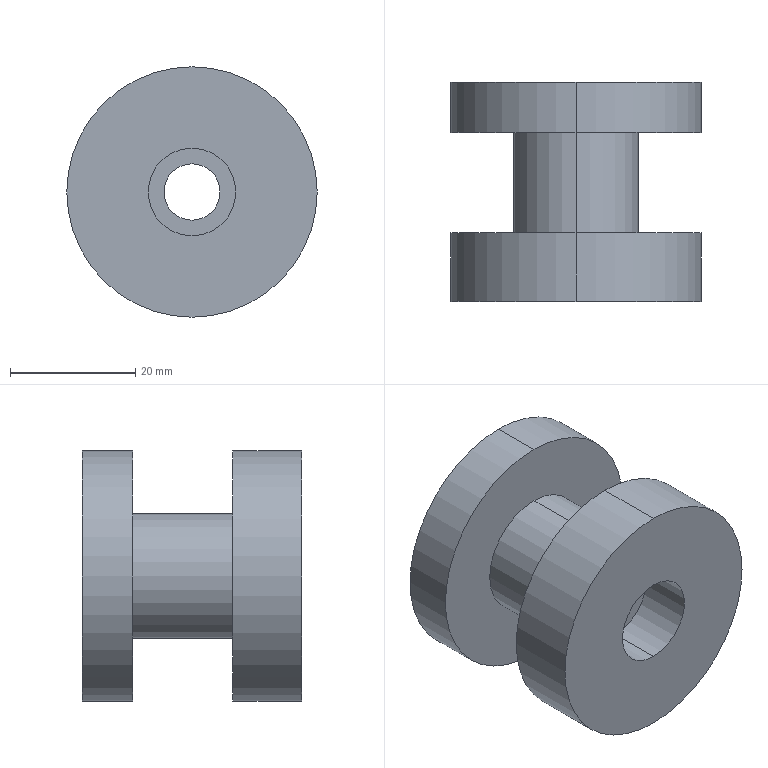Part | STEP file | 0229_206_Joint | 1 solid | 20 faces | box 40 x 35 x 40 mm | volume 25414 mm3 | cylinder 12 | plane 6 | cone 2 | commonest cylinder face diameters 40 x4 9 x2 14 x2 16.6 x2 20 x2
STEP:
#1=CARTESIAN_POINT('',(0.,0.,0.));
#2=DIRECTION('',(0.,0.,1.));
#3=DIRECTION('',(1.,0.,0.));
#4=AXIS2_PLACEMENT_3D('',#1,#2,#3);
#5=CARTESIAN_POINT('',(0.,2.,8.3));
#6=VERTEX_POINT('',#5);
#7=CARTESIAN_POINT('',(0.,3.,9.3));
#8=VERTEX_POINT('',#7);
#9=CARTESIAN_POINT('',(0.,3.,9.3));
#10=DIRECTION('',(0.,0.7071,0.7071));
#11=VECTOR('',#10,1.);
#12=LINE('',#9,#11);
#13=CARTESIAN_POINT('',(0.,3.,0.));
#14=DIRECTION('',(0.,1.,0.));
#15=DIRECTION('',(0.,0.,1.));
#16=AXIS2_PLACEMENT_3D('',#13,#14,#15);
#17=CONICAL_SURFACE('',#16,9.3,0.7854);
#18=CARTESIAN_POINT('',(6.283,0.));
#19=DIRECTION('',(0.,1.));
#20=VECTOR('',#19,1.);
#21=LINE('',#18,#20);
#22=(GEOMETRIC_REPRESENTATION_CONTEXT(2)PARAMETRIC_REPRESENTATION_CONTEXT()REPRESENTATION_CONTEXT('',''));
#23=DEFINITIONAL_REPRESENTATION('',(#21),#22);
#24=PCURVE('',#17,#23);
#25=CARTESIAN_POINT('',(0.,3.,0.));
#26=DIRECTION('',(0.,1.,0.));
#27=DIRECTION('',(0.,0.,1.));
#28=AXIS2_PLACEMENT_3D('',#25,#26,#27);
#29=CONICAL_SURFACE('',#28,9.3,0.7854);
#30=CARTESIAN_POINT('',(0.,0.));
#31=DIRECTION('',(0.,1.));
#32=VECTOR('',#31,1.);
#33=LINE('',#30,#32);
#34=(GEOMETRIC_REPRESENTATION_CONTEXT(2)PARAMETRIC_REPRESENTATION_CONTEXT()REPRESENTATION_CONTEXT('',''));
#35=DEFINITIONAL_REPRESENTATION('',(#33),#34);
#36=PCURVE('',#29,#35);
#37=SURFACE_CURVE('',#12,(#24,#36),.PCURVE_S1.);
#38=EDGE_CURVE('',#6,#8,#37,.T.);
#39=ORIENTED_EDGE('',*,*,#38,.T.);
#40=CARTESIAN_POINT('',(0.,3.,-9.3));
#41=VERTEX_POINT('',#40);
#42=CARTESIAN_POINT('',(0.,3.,0.));
#43=DIRECTION('',(0.,-1.,0.));
#44=DIRECTION('',(0.,0.,-1.));
#45=AXIS2_PLACEMENT_3D('',#42,#43,#44);
#46=CIRCLE('',#45,9.3);
#47=CARTESIAN_POINT('',(9.425,0.));
#48=DIRECTION('',(-1.,0.));
#49=VECTOR('',#48,1.);
#50=LINE('',#47,#49);
#51=(GEOMETRIC_REPRESENTATION_CONTEXT(2)PARAMETRIC_REPRESENTATION_CONTEXT()REPRESENTATION_CONTEXT('',''));
#52=DEFINITIONAL_REPRESENTATION('',(#50),#51);
#53=PCURVE('',#17,#52);
#54=CARTESIAN_POINT('',(0.,3.,0.));
#55=DIRECTION('',(0.,-1.,0.));
#56=DIRECTION('',(0.,0.,-1.));
#57=AXIS2_PLACEMENT_3D('',#54,#55,#56);
#58=PLANE('',#57);
#59=CARTESIAN_POINT('',(0.,0.));
#60=DIRECTION('',(1.,0.));
#61=AXIS2_PLACEMENT_2D('',#59,#60);
#62=CIRCLE('',#61,9.3);
#63=(GEOMETRIC_REPRESENTATION_CONTEXT(2)PARAMETRIC_REPRESENTATION_CONTEXT()REPRESENTATION_CONTEXT('',''));
#64=DEFINITIONAL_REPRESENTATION('',(#62),#63);
#65=PCURVE('',#58,#64);
#66=SURFACE_CURVE('',#46,(#53,#65),.PCURVE_S1.);
#67=EDGE_CURVE('',#8,#41,#66,.T.);
#68=ORIENTED_EDGE('',*,*,#67,.T.);
#69=CARTESIAN_POINT('',(0.,2.,-8.3));
#70=VERTEX_POINT('',#69);
#71=CARTESIAN_POINT('',(0.,3.,-9.3));
#72=DIRECTION('',(0.,0.7071,-0.7071));
#73=VECTOR('',#72,1.);
#74=LINE('',#71,#73);
#75=CARTESIAN_POINT('',(3.142,0.));
#76=DIRECTION('',(0.,1.));
#77=VECTOR('',#76,1.);
#78=LINE('',#75,#77);
#79=(GEOMETRIC_REPRESENTATION_CONTEXT(2)PARAMETRIC_REPRESENTATION_CONTEXT()REPRESENTATION_CONTEXT('',''));
#80=DEFINITIONAL_REPRESENTATION('',(#78),#79);
#81=PCURVE('',#17,#80);
#82=CARTESIAN_POINT('',(3.142,0.));
#83=DIRECTION('',(0.,1.));
#84=VECTOR('',#83,1.);
#85=LINE('',#82,#84);
#86=(GEOMETRIC_REPRESENTATION_CONTEXT(2)PARAMETRIC_REPRESENTATION_CONTEXT()REPRESENTATION_CONTEXT('',''));
#87=DEFINITIONAL_REPRESENTATION('',(#85),#86);
#88=PCURVE('',#29,#87);
#89=SURFACE_CURVE('',#74,(#81,#88),.PCURVE_S1.);
#90=EDGE_CURVE('',#70,#41,#89,.T.);
#91=ORIENTED_EDGE('',*,*,#90,.F.);
#92=CARTESIAN_POINT('',(0.,2.,0.));
#93=DIRECTION('',(0.,1.,0.));
#94=DIRECTION('',(0.,0.,-1.));
#95=AXIS2_PLACEMENT_3D('',#92,#93,#94);
#96=CIRCLE('',#95,8.3);
#97=CARTESIAN_POINT('',(3.142,-1.));
#98=DIRECTION('',(1.,0.));
#99=VECTOR('',#98,1.);
#100=LINE('',#97,#99);
#101=(GEOMETRIC_REPRESENTATION_CONTEXT(2)PARAMETRIC_REPRESENTATION_CONTEXT()REPRESENTATION_CONTEXT('',''));
#102=DEFINITIONAL_REPRESENTATION('',(#100),#101);
#103=PCURVE('',#17,#102);
#104=CARTESIAN_POINT('',(0.,-3.154,0.));
#105=DIRECTION('',(0.,-1.,0.));
#106=DIRECTION('',(0.,0.,-1.));
#107=AXIS2_PLACEMENT_3D('',#104,#105,#106);
#108=CYLINDRICAL_SURFACE('',#107,8.3);
#109=CARTESIAN_POINT('',(6.283,-5.154));
#110=DIRECTION('',(-1.,0.));
#111=VECTOR('',#110,1.);
#112=LINE('',#109,#111);
#113=(GEOMETRIC_REPRESENTATION_CONTEXT(2)PARAMETRIC_REPRESENTATION_CONTEXT()REPRESENTATION_CONTEXT('',''));
#114=DEFINITIONAL_REPRESENTATION('',(#112),#113);
#115=PCURVE('',#108,#114);
#116=SURFACE_CURVE('',#96,(#103,#115),.PCURVE_S1.);
#117=EDGE_CURVE('',#70,#6,#116,.T.);
#118=ORIENTED_EDGE('',*,*,#117,.T.);
#119=EDGE_LOOP('',(#39,#68,#91,#118));
#120=FACE_BOUND('',#119,.F.);
#121=ADVANCED_FACE('',(#120),#17,.F.);
#122=CARTESIAN_POINT('',(0.,-23.4,-7.));
#123=VERTEX_POINT('',#122);
#124=CARTESIAN_POINT('',(0.,-32.,-7.));
#125=VERTEX_POINT('',#124);
#126=CARTESIAN_POINT('',(0.,-32.,-7.));
#127=DIRECTION('',(0.,-1.,0.));
#128=VECTOR('',#127,1.);
#129=LINE('',#126,#128);
#130=CARTESIAN_POINT('',(0.,-32.,0.));
#131=DIRECTION('',(0.,-1.,0.));
#132=DIRECTION('',(0.,0.,-1.));
#133=AXIS2_PLACEMENT_3D('',#130,#131,#132);
#134=CYLINDRICAL_SURFACE('',#133,7.);
#135=CARTESIAN_POINT('',(6.283,0.));
#136=DIRECTION('',(0.,1.));
#137=VECTOR('',#136,1.);
#138=LINE('',#135,#137);
#139=(GEOMETRIC_REPRESENTATION_CONTEXT(2)PARAMETRIC_REPRESENTATION_CONTEXT()REPRESENTATION_CONTEXT('',''));
#140=DEFINITIONAL_REPRESENTATION('',(#138),#139);
#141=PCURVE('',#134,#140);
#142=CARTESIAN_POINT('',(0.,-32.,0.));
#143=DIRECTION('',(0.,-1.,0.));
#144=DIRECTION('',(0.,0.,-1.));
#145=AXIS2_PLACEMENT_3D('',#142,#143,#144);
#146=CYLINDRICAL_SURFACE('',#145,7.);
#147=CARTESIAN_POINT('',(0.,0.));
#148=DIRECTION('',(0.,1.));
#149=VECTOR('',#148,1.);
#150=LINE('',#147,#149);
#151=(GEOMETRIC_REPRESENTATION_CONTEXT(2)PARAMETRIC_REPRESENTATION_CONTEXT()REPRESENTATION_CONTEXT('',''));
#152=DEFINITIONAL_REPRESENTATION('',(#150),#151);
#153=PCURVE('',#146,#152);
#154=SURFACE_CURVE('',#129,(#141,#153),.PCURVE_S1.);
#155=EDGE_CURVE('',#123,#125,#154,.T.);
#156=ORIENTED_EDGE('',*,*,#155,.T.);
#157=CARTESIAN_POINT('',(0.,-32.,7.));
#158=VERTEX_POINT('',#157);
#159=CARTESIAN_POINT('',(0.,-32.,0.));
#160=DIRECTION('',(0.,-1.,0.));
#161=DIRECTION('',(0.,0.,-1.));
#162=AXIS2_PLACEMENT_3D('',#159,#160,#161);
#163=CIRCLE('',#162,7.);
#164=CARTESIAN_POINT('',(0.,0.));
#165=DIRECTION('',(1.,0.));
#166=VECTOR('',#165,1.);
#167=LINE('',#164,#166);
#168=(GEOMETRIC_REPRESENTATION_CONTEXT(2)PARAMETRIC_REPRESENTATION_CONTEXT()REPRESENTATION_CONTEXT('',''));
#169=DEFINITIONAL_REPRESENTATION('',(#167),#168);
#170=PCURVE('',#134,#169);
#171=CARTESIAN_POINT('',(-20.,-32.,0.));
#172=DIRECTION('',(0.,1.,0.));
#173=DIRECTION('',(0.,0.,1.));
#174=AXIS2_PLACEMENT_3D('',#171,#172,#173);
#175=PLANE('',#174);
#176=CARTESIAN_POINT('',(-7.,20.));
#177=CARTESIAN_POINT('',(-7.,32.124));
#178=CARTESIAN_POINT('',(3.5,26.062));
#179=CARTESIAN_POINT('',(14.,20.));
#180=CARTESIAN_POINT('',(3.5,13.938));
#181=CARTESIAN_POINT('',(-7.,7.876));
#182=CARTESIAN_POINT('',(-7.,20.));
#183=(BOUNDED_CURVE()B_SPLINE_CURVE(2,(#176,#177,#178,#179,#180,#181,#182),.UNSPECIFIED.,.T.,.F.)B_SPLINE_CURVE_WITH_KNOTS((1,2,2,2,2,1),(-2.094,0.,2.094,4.189,6.283,8.378),.UNSPECIFIED.)CURVE()GEOMETRIC_REPRESENTATION_ITEM()RATIONAL_B_SPLINE_CURVE((1.,0.5,1.,0.5,1.,0.5,1.))REPRESENTATION_ITEM(''));
#184=(GEOMETRIC_REPRESENTATION_CONTEXT(2)PARAMETRIC_REPRESENTATION_CONTEXT()REPRESENTATION_CONTEXT('',''));
#185=DEFINITIONAL_REPRESENTATION('',(#183),#184);
#186=PCURVE('',#175,#185);
#187=SURFACE_CURVE('',#163,(#170,#186),.PCURVE_S1.);
#188=EDGE_CURVE('',#158,#125,#187,.T.);
#189=ORIENTED_EDGE('',*,*,#188,.F.);
#190=CARTESIAN_POINT('',(0.,-23.4,7.));
#191=VERTEX_POINT('',#190);
#192=CARTESIAN_POINT('',(0.,-32.,7.));
#193=DIRECTION('',(0.,-1.,0.));
#194=VECTOR('',#193,1.);
#195=LINE('',#192,#194);
#196=CARTESIAN_POINT('',(3.142,0.));
#197=DIRECTION('',(0.,1.));
#198=VECTOR('',#197,1.);
#199=LINE('',#196,#198);
#200=(GEOMETRIC_REPRESENTATION_CONTEXT(2)PARAMETRIC_REPRESENTATION_CONTEXT()REPRESENTATION_CONTEXT('',''));
#201=DEFINITIONAL_REPRESENTATION('',(#199),#200);
#202=PCURVE('',#134,#201);
#203=CARTESIAN_POINT('',(3.142,0.));
#204=DIRECTION('',(0.,1.));
#205=VECTOR('',#204,1.);
#206=LINE('',#203,#205);
#207=(GEOMETRIC_REPRESENTATION_CONTEXT(2)PARAMETRIC_REPRESENTATION_CONTEXT()REPRESENTATION_CONTEXT('',''));
#208=DEFINITIONAL_REPRESENTATION('',(#206),#207);
#209=PCURVE('',#146,#208);
#210=SURFACE_CURVE('',#195,(#202,#209),.PCURVE_S1.);
#211=EDGE_CURVE('',#191,#158,#210,.T.);
#212=ORIENTED_EDGE('',*,*,#211,.F.);
#213=CARTESIAN_POINT('',(0.,-23.4,0.));
#214=DIRECTION('',(0.,-1.,0.));
#215=DIRECTION('',(0.,0.,-1.));
#216=AXIS2_PLACEMENT_3D('',#213,#214,#215);
#217=CIRCLE('',#216,7.);
#218=CARTESIAN_POINT('',(0.,-8.6));
#219=DIRECTION('',(1.,0.));
#220=VECTOR('',#219,1.);
#221=LINE('',#218,#220);
#222=(GEOMETRIC_REPRESENTATION_CONTEXT(2)PARAMETRIC_REPRESENTATION_CONTEXT()REPRESENTATION_CONTEXT('',''));
#223=DEFINITIONAL_REPRESENTATION('',(#221),#222);
#224=PCURVE('',#134,#223);
#225=CARTESIAN_POINT('',(4.5,-23.4,0.));
#226=DIRECTION('',(0.,1.,0.));
#227=DIRECTION('',(0.,0.,1.));
#228=AXIS2_PLACEMENT_3D('',#225,#226,#227);
#229=PLANE('',#228);
#230=CARTESIAN_POINT('',(-7.,-4.5));
#231=CARTESIAN_POINT('',(-7.,7.624));
#232=CARTESIAN_POINT('',(3.5,1.562));
#233=CARTESIAN_POINT('',(14.,-4.5));
#234=CARTESIAN_POINT('',(3.5,-10.562));
#235=CARTESIAN_POINT('',(-7.,-16.624));
#236=CARTESIAN_POINT('',(-7.,-4.5));
#237=(BOUNDED_CURVE()B_SPLINE_CURVE(2,(#230,#231,#232,#233,#234,#235,#236),.UNSPECIFIED.,.T.,.F.)B_SPLINE_CURVE_WITH_KNOTS((1,2,2,2,2,1),(-2.094,0.,2.094,4.189,6.283,8.378),.UNSPECIFIED.)CURVE()GEOMETRIC_REPRESENTATION_ITEM()RATIONAL_B_SPLINE_CURVE((1.,0.5,1.,0.5,1.,0.5,1.))REPRESENTATION_ITEM(''));
#238=(GEOMETRIC_REPRESENTATION_CONTEXT(2)PARAMETRIC_REPRESENTATION_CONTEXT()REPRESENTATION_CONTEXT('',''));
#239=DEFINITIONAL_REPRESENTATION('',(#237),#238);
#240=PCURVE('',#229,#239);
#241=SURFACE_CURVE('',#217,(#224,#240),.PCURVE_S1.);
#242=EDGE_CURVE('',#191,#123,#241,.T.);
#243=ORIENTED_EDGE('',*,*,#242,.T.);
#244=EDGE_LOOP('',(#156,#189,#212,#243));
#245=FACE_BOUND('',#244,.F.);
#246=ADVANCED_FACE('',(#245),#134,.F.);
#247=CARTESIAN_POINT('',(0.,0.,-4.5));
#248=VERTEX_POINT('',#247);
#249=CARTESIAN_POINT('',(0.,-23.4,-4.5));
#250=VERTEX_POINT('',#249);
#251=CARTESIAN_POINT('',(0.,-32.,-4.5));
#252=DIRECTION('',(0.,-1.,0.));
#253=VECTOR('',#252,1.);
#254=LINE('',#251,#253);
#255=CARTESIAN_POINT('',(0.,-32.,0.));
#256=DIRECTION('',(0.,-1.,0.));
#257=DIRECTION('',(0.,0.,-1.));
#258=AXIS2_PLACEMENT_3D('',#255,#256,#257);
#259=CYLINDRICAL_SURFACE('',#258,4.5);
#260=CARTESIAN_POINT('',(6.283,0.));
#261=DIRECTION('',(0.,1.));
#262=VECTOR('',#261,1.);
#263=LINE('',#260,#262);
#264=(GEOMETRIC_REPRESENTATION_CONTEXT(2)PARAMETRIC_REPRESENTATION_CONTEXT()REPRESENTATION_CONTEXT('',''));
#265=DEFINITIONAL_REPRESENTATION('',(#263),#264);
#266=PCURVE('',#259,#265);
#267=CARTESIAN_POINT('',(0.,-32.,0.));
#268=DIRECTION('',(0.,-1.,0.));
#269=DIRECTION('',(0.,0.,-1.));
#270=AXIS2_PLACEMENT_3D('',#267,#268,#269);
#271=CYLINDRICAL_SURFACE('',#270,4.5);
#272=CARTESIAN_POINT('',(0.,0.));
#273=DIRECTION('',(0.,1.));
#274=VECTOR('',#273,1.);
#275=LINE('',#272,#274);
#276=(GEOMETRIC_REPRESENTATION_CONTEXT(2)PARAMETRIC_REPRESENTATION_CONTEXT()REPRESENTATION_CONTEXT('',''));
#277=DEFINITIONAL_REPRESENTATION('',(#275),#276);
#278=PCURVE('',#271,#277);
#279=SURFACE_CURVE('',#254,(#266,#278),.PCURVE_S1.);
#280=EDGE_CURVE('',#248,#250,#279,.T.);
#281=ORIENTED_EDGE('',*,*,#280,.T.);
#282=CARTESIAN_POINT('',(0.,-23.4,4.5));
#283=VERTEX_POINT('',#282);
#284=CARTESIAN_POINT('',(0.,-23.4,0.));
#285=DIRECTION('',(0.,-1.,0.));
#286=DIRECTION('',(0.,0.,-1.));
#287=AXIS2_PLACEMENT_3D('',#284,#285,#286);
#288=CIRCLE('',#287,4.5);
#289=CARTESIAN_POINT('',(0.,-8.6));
#290=DIRECTION('',(1.,0.));
#291=VECTOR('',#290,1.);
#292=LINE('',#289,#291);
#293=(GEOMETRIC_REPRESENTATION_CONTEXT(2)PARAMETRIC_REPRESENTATION_CONTEXT()REPRESENTATION_CONTEXT('',''));
#294=DEFINITIONAL_REPRESENTATION('',(#292),#293);
#295=PCURVE('',#259,#294);
#296=CARTESIAN_POINT('',(-4.5,-4.5));
#297=CARTESIAN_POINT('',(-4.5,3.294));
#298=CARTESIAN_POINT('',(2.25,-0.6029));
#299=CARTESIAN_POINT('',(9.,-4.5));
#300=CARTESIAN_POINT('',(2.25,-8.397));
#301=CARTESIAN_POINT('',(-4.5,-12.294));
#302=CARTESIAN_POINT('',(-4.5,-4.5));
#303=(BOUNDED_CURVE()B_SPLINE_CURVE(2,(#296,#297,#298,#299,#300,#301,#302),.UNSPECIFIED.,.T.,.F.)B_SPLINE_CURVE_WITH_KNOTS((1,2,2,2,2,1),(-2.094,0.,2.094,4.189,6.283,8.378),.UNSPECIFIED.)CURVE()GEOMETRIC_REPRESENTATION_ITEM()RATIONAL_B_SPLINE_CURVE((1.,0.5,1.,0.5,1.,0.5,1.))REPRESENTATION_ITEM(''));
#304=(GEOMETRIC_REPRESENTATION_CONTEXT(2)PARAMETRIC_REPRESENTATION_CONTEXT()REPRESENTATION_CONTEXT('',''));
#305=DEFINITIONAL_REPRESENTATION('',(#303),#304);
#306=PCURVE('',#229,#305);
#307=SURFACE_CURVE('',#288,(#295,#306),.PCURVE_S1.);
#308=EDGE_CURVE('',#283,#250,#307,.T.);
#309=ORIENTED_EDGE('',*,*,#308,.F.);
#310=CARTESIAN_POINT('',(0.,0.,4.5));
#311=VERTEX_POINT('',#310);
#312=CARTESIAN_POINT('',(0.,-32.,4.5));
#313=DIRECTION('',(0.,-1.,0.));
#314=VECTOR('',#313,1.);
#315=LINE('',#312,#314);
#316=CARTESIAN_POINT('',(3.142,0.));
#317=DIRECTION('',(0.,1.));
#318=VECTOR('',#317,1.);
#319=LINE('',#316,#318);
#320=(GEOMETRIC_REPRESENTATION_CONTEXT(2)PARAMETRIC_REPRESENTATION_CONTEXT()REPRESENTATION_CONTEXT('',''));
#321=DEFINITIONAL_REPRESENTATION('',(#319),#320);
#322=PCURVE('',#259,#321);
#323=CARTESIAN_POINT('',(3.142,0.));
#324=DIRECTION('',(0.,1.));
#325=VECTOR('',#324,1.);
#326=LINE('',#323,#325);
#327=(GEOMETRIC_REPRESENTATION_CONTEXT(2)PARAMETRIC_REPRESENTATION_CONTEXT()REPRESENTATION_CONTEXT('',''));
#328=DEFINITIONAL_REPRESENTATION('',(#326),#327);
#329=PCURVE('',#271,#328);
#330=SURFACE_CURVE('',#315,(#322,#329),.PCURVE_S1.);
#331=EDGE_CURVE('',#311,#283,#330,.T.);
#332=ORIENTED_EDGE('',*,*,#331,.F.);
#333=CARTESIAN_POINT('',(0.,0.,0.));
#334=DIRECTION('',(0.,1.,0.));
#335=DIRECTION('',(0.,0.,1.));
#336=AXIS2_PLACEMENT_3D('',#333,#334,#335);
#337=CIRCLE('',#336,4.5);
#338=CARTESIAN_POINT('',(9.425,-32.));
#339=DIRECTION('',(-1.,0.));
#340=VECTOR('',#339,1.);
#341=LINE('',#338,#340);
#342=(GEOMETRIC_REPRESENTATION_CONTEXT(2)PARAMETRIC_REPRESENTATION_CONTEXT()REPRESENTATION_CONTEXT('',''));
#343=DEFINITIONAL_REPRESENTATION('',(#341),#342);
#344=PCURVE('',#259,#343);
#345=CARTESIAN_POINT('',(0.,0.,0.));
#346=DIRECTION('',(0.,1.,0.));
#347=DIRECTION('',(0.,0.,1.));
#348=AXIS2_PLACEMENT_3D('',#345,#346,#347);
#349=PLANE('',#348);
#350=CARTESIAN_POINT('',(0.,0.));
#351=DIRECTION('',(1.,0.));
#352=AXIS2_PLACEMENT_2D('',#350,#351);
#353=CIRCLE('',#352,4.5);
#354=(GEOMETRIC_REPRESENTATION_CONTEXT(2)PARAMETRIC_REPRESENTATION_CONTEXT()REPRESENTATION_CONTEXT('',''));
#355=DEFINITIONAL_REPRESENTATION('',(#353),#354);
#356=PCURVE('',#349,#355);
#357=SURFACE_CURVE('',#337,(#344,#356),.PCURVE_S1.);
#358=EDGE_CURVE('',#248,#311,#357,.T.);
#359=ORIENTED_EDGE('',*,*,#358,.F.);
#360=EDGE_LOOP('',(#281,#309,#332,#359));
#361=FACE_BOUND('',#360,.F.);
#362=ADVANCED_FACE('',(#361),#259,.F.);
#363=CARTESIAN_POINT('',(0.,0.,-8.3));
#364=VERTEX_POINT('',#363);
#365=CARTESIAN_POINT('',(0.,-3.154,-8.3));
#366=DIRECTION('',(0.,-1.,0.));
#367=VECTOR('',#366,1.);
#368=LINE('',#365,#367);
#369=CARTESIAN_POINT('',(6.283,0.));
#370=DIRECTION('',(0.,1.));
#371=VECTOR('',#370,1.);
#372=LINE('',#369,#371);
#373=(GEOMETRIC_REPRESENTATION_CONTEXT(2)PARAMETRIC_REPRESENTATION_CONTEXT()REPRESENTATION_CONTEXT('',''));
#374=DEFINITIONAL_REPRESENTATION('',(#372),#373);
#375=PCURVE('',#108,#374);
#376=CARTESIAN_POINT('',(0.,-3.154,0.));
#377=DIRECTION('',(0.,-1.,0.));
#378=DIRECTION('',(0.,0.,-1.));
#379=AXIS2_PLACEMENT_3D('',#376,#377,#378);
#380=CYLINDRICAL_SURFACE('',#379,8.3);
#381=CARTESIAN_POINT('',(0.,0.));
#382=DIRECTION('',(0.,1.));
#383=VECTOR('',#382,1.);
#384=LINE('',#381,#383);
#385=(GEOMETRIC_REPRESENTATION_CONTEXT(2)PARAMETRIC_REPRESENTATION_CONTEXT()REPRESENTATION_CONTEXT('',''));
#386=DEFINITIONAL_REPRESENTATION('',(#384),#385);
#387=PCURVE('',#380,#386);
#388=SURFACE_CURVE('',#368,(#375,#387),.PCURVE_S1.);
#389=EDGE_CURVE('',#70,#364,#388,.T.);
#390=ORIENTED_EDGE('',*,*,#389,.T.);
#391=CARTESIAN_POINT('',(0.,0.,8.3));
#392=VERTEX_POINT('',#391);
#393=CARTESIAN_POINT('',(0.,0.,0.));
#394=DIRECTION('',(0.,-1.,0.));
#395=DIRECTION('',(0.,0.,-1.));
#396=AXIS2_PLACEMENT_3D('',#393,#394,#395);
#397=CIRCLE('',#396,8.3);
#398=CARTESIAN_POINT('',(0.,-3.154));
#399=DIRECTION('',(1.,0.));
#400=VECTOR('',#399,1.);
#401=LINE('',#398,#400);
#402=(GEOMETRIC_REPRESENTATION_CONTEXT(2)PARAMETRIC_REPRESENTATION_CONTEXT()REPRESENTATION_CONTEXT('',''));
#403=DEFINITIONAL_REPRESENTATION('',(#401),#402);
#404=PCURVE('',#108,#403);
#405=CARTESIAN_POINT('',(-8.3,0.));
#406=CARTESIAN_POINT('',(-8.3,14.376));
#407=CARTESIAN_POINT('',(4.15,7.188));
#408=CARTESIAN_POINT('',(16.6,0.));
#409=CARTESIAN_POINT('',(4.15,-7.188));
#410=CARTESIAN_POINT('',(-8.3,-14.376));
#411=CARTESIAN_POINT('',(-8.3,0.));
#412=(BOUNDED_CURVE()B_SPLINE_CURVE(2,(#405,#406,#407,#408,#409,#410,#411),.UNSPECIFIED.,.T.,.F.)B_SPLINE_CURVE_WITH_KNOTS((1,2,2,2,2,1),(-2.094,0.,2.094,4.189,6.283,8.378),.UNSPECIFIED.)CURVE()GEOMETRIC_REPRESENTATION_ITEM()RATIONAL_B_SPLINE_CURVE((1.,0.5,1.,0.5,1.,0.5,1.))REPRESENTATION_ITEM(''));
#413=(GEOMETRIC_REPRESENTATION_CONTEXT(2)PARAMETRIC_REPRESENTATION_CONTEXT()REPRESENTATION_CONTEXT('',''));
#414=DEFINITIONAL_REPRESENTATION('',(#412),#413);
#415=PCURVE('',#349,#414);
#416=SURFACE_CURVE('',#397,(#404,#415),.PCURVE_S1.);
#417=EDGE_CURVE('',#392,#364,#416,.T.);
#418=ORIENTED_EDGE('',*,*,#417,.F.);
#419=CARTESIAN_POINT('',(0.,-3.154,8.3));
#420=DIRECTION('',(0.,-1.,0.));
#421=VECTOR('',#420,1.);
#422=LINE('',#419,#421);
#423=CARTESIAN_POINT('',(3.142,0.));
#424=DIRECTION('',(0.,1.));
#425=VECTOR('',#424,1.);
#426=LINE('',#423,#425);
#427=(GEOMETRIC_REPRESENTATION_CONTEXT(2)PARAMETRIC_REPRESENTATION_CONTEXT()REPRESENTATION_CONTEXT('',''));
#428=DEFINITIONAL_REPRESENTATION('',(#426),#427);
#429=PCURVE('',#108,#428);
#430=CARTESIAN_POINT('',(3.142,0.));
#431=DIRECTION('',(0.,1.));
#432=VECTOR('',#431,1.);
#433=LINE('',#430,#432);
#434=(GEOMETRIC_REPRESENTATION_CONTEXT(2)PARAMETRIC_REPRESENTATION_CONTEXT()REPRESENTATION_CONTEXT('',''));
#435=DEFINITIONAL_REPRESENTATION('',(#433),#434);
#436=PCURVE('',#380,#435);
#437=SURFACE_CURVE('',#422,(#429,#436),.PCURVE_S1.);
#438=EDGE_CURVE('',#6,#392,#437,.T.);
#439=ORIENTED_EDGE('',*,*,#438,.F.);
#440=ORIENTED_EDGE('',*,*,#117,.F.);
#441=EDGE_LOOP('',(#390,#418,#439,#440));
#442=FACE_BOUND('',#441,.F.);
#443=ADVANCED_FACE('',(#442),#108,.F.);
#444=CARTESIAN_POINT('',(0.,-21.,-20.));
#445=VERTEX_POINT('',#444);
#446=CARTESIAN_POINT('',(0.,-21.,20.));
#447=VERTEX_POINT('',#446);
#448=CARTESIAN_POINT('',(0.,-21.,0.));
#449=DIRECTION('',(0.,-1.,0.));
#450=DIRECTION('',(0.,0.,-1.));
#451=AXIS2_PLACEMENT_3D('',#448,#449,#450);
#452=CIRCLE('',#451,20.);
#453=CARTESIAN_POINT('',(0.,-64.451,0.));
#454=DIRECTION('',(0.,-1.,0.));
#455=DIRECTION('',(0.,0.,-1.));
#456=AXIS2_PLACEMENT_3D('',#453,#454,#455);
#457=CYLINDRICAL_SURFACE('',#456,20.);
#458=CARTESIAN_POINT('',(0.,-43.451));
#459=DIRECTION('',(1.,0.));
#460=VECTOR('',#459,1.);
#461=LINE('',#458,#460);
#462=(GEOMETRIC_REPRESENTATION_CONTEXT(2)PARAMETRIC_REPRESENTATION_CONTEXT()REPRESENTATION_CONTEXT('',''));
#463=DEFINITIONAL_REPRESENTATION('',(#461),#462);
#464=PCURVE('',#457,#463);
#465=CARTESIAN_POINT('',(-10.,-21.,0.));
#466=DIRECTION('',(0.,-1.,0.));
#467=DIRECTION('',(0.,0.,-1.));
#468=AXIS2_PLACEMENT_3D('',#465,#466,#467);
#469=PLANE('',#468);
#470=CARTESIAN_POINT('',(0.,10.));
#471=DIRECTION('',(1.,0.));
#472=AXIS2_PLACEMENT_2D('',#470,#471);
#473=CIRCLE('',#472,20.);
#474=(GEOMETRIC_REPRESENTATION_CONTEXT(2)PARAMETRIC_REPRESENTATION_CONTEXT()REPRESENTATION_CONTEXT('',''));
#475=DEFINITIONAL_REPRESENTATION('',(#473),#474);
#476=PCURVE('',#469,#475);
#477=SURFACE_CURVE('',#452,(#464,#476),.PCURVE_S1.);
#478=EDGE_CURVE('',#445,#447,#477,.T.);
#479=ORIENTED_EDGE('',*,*,#478,.T.);
#480=CARTESIAN_POINT('',(0.,-32.,20.));
#481=VERTEX_POINT('',#480);
#482=CARTESIAN_POINT('',(0.,-64.451,20.));
#483=DIRECTION('',(0.,-1.,0.));
#484=VECTOR('',#483,1.);
#485=LINE('',#482,#484);
#486=CARTESIAN_POINT('',(3.142,0.));
#487=DIRECTION('',(0.,1.));
#488=VECTOR('',#487,1.);
#489=LINE('',#486,#488);
#490=(GEOMETRIC_REPRESENTATION_CONTEXT(2)PARAMETRIC_REPRESENTATION_CONTEXT()REPRESENTATION_CONTEXT('',''));
#491=DEFINITIONAL_REPRESENTATION('',(#489),#490);
#492=PCURVE('',#457,#491);
#493=CARTESIAN_POINT('',(0.,-64.451,0.));
#494=DIRECTION('',(0.,-1.,0.));
#495=DIRECTION('',(0.,0.,-1.));
#496=AXIS2_PLACEMENT_3D('',#493,#494,#495);
#497=CYLINDRICAL_SURFACE('',#496,20.);
#498=CARTESIAN_POINT('',(3.142,0.));
#499=DIRECTION('',(0.,1.));
#500=VECTOR('',#499,1.);
#501=LINE('',#498,#500);
#502=(GEOMETRIC_REPRESENTATION_CONTEXT(2)PARAMETRIC_REPRESENTATION_CONTEXT()REPRESENTATION_CONTEXT('',''));
#503=DEFINITIONAL_REPRESENTATION('',(#501),#502);
#504=PCURVE('',#497,#503);
#505=SURFACE_CURVE('',#485,(#492,#504),.PCURVE_S1.);
#506=EDGE_CURVE('',#447,#481,#505,.T.);
#507=ORIENTED_EDGE('',*,*,#506,.T.);
#508=CARTESIAN_POINT('',(0.,-32.,-20.));
#509=VERTEX_POINT('',#508);
#510=CARTESIAN_POINT('',(0.,-32.,0.));
#511=DIRECTION('',(0.,-1.,0.));
#512=DIRECTION('',(0.,0.,-1.));
#513=AXIS2_PLACEMENT_3D('',#510,#511,#512);
#514=CIRCLE('',#513,20.);
#515=CARTESIAN_POINT('',(0.,-32.451));
#516=DIRECTION('',(1.,0.));
#517=VECTOR('',#516,1.);
#518=LINE('',#515,#517);
#519=(GEOMETRIC_REPRESENTATION_CONTEXT(2)PARAMETRIC_REPRESENTATION_CONTEXT()REPRESENTATION_CONTEXT('',''));
#520=DEFINITIONAL_REPRESENTATION('',(#518),#519);
#521=PCURVE('',#457,#520);
#522=CARTESIAN_POINT('',(-20.,20.));
#523=CARTESIAN_POINT('',(-20.,54.641));
#524=CARTESIAN_POINT('',(10.,37.321));
#525=CARTESIAN_POINT('',(40.,20.));
#526=CARTESIAN_POINT('',(10.,2.679));
#527=CARTESIAN_POINT('',(-20.,-14.641));
#528=CARTESIAN_POINT('',(-20.,20.));
#529=(BOUNDED_CURVE()B_SPLINE_CURVE(2,(#522,#523,#524,#525,#526,#527,#528),.UNSPECIFIED.,.T.,.F.)B_SPLINE_CURVE_WITH_KNOTS((1,2,2,2,2,1),(-2.094,0.,2.094,4.189,6.283,8.378),.UNSPECIFIED.)CURVE()GEOMETRIC_REPRESENTATION_ITEM()RATIONAL_B_SPLINE_CURVE((1.,0.5,1.,0.5,1.,0.5,1.))REPRESENTATION_ITEM(''));
#530=(GEOMETRIC_REPRESENTATION_CONTEXT(2)PARAMETRIC_REPRESENTATION_CONTEXT()REPRESENTATION_CONTEXT('',''));
#531=DEFINITIONAL_REPRESENTATION('',(#529),#530);
#532=PCURVE('',#175,#531);
#533=SURFACE_CURVE('',#514,(#521,#532),.PCURVE_S1.);
#534=EDGE_CURVE('',#509,#481,#533,.T.);
#535=ORIENTED_EDGE('',*,*,#534,.F.);
#536=CARTESIAN_POINT('',(0.,-64.451,-20.));
#537=DIRECTION('',(0.,-1.,0.));
#538=VECTOR('',#537,1.);
#539=LINE('',#536,#538);
#540=CARTESIAN_POINT('',(0.,0.));
#541=DIRECTION('',(0.,1.));
#542=VECTOR('',#541,1.);
#543=LINE('',#540,#542);
#544=(GEOMETRIC_REPRESENTATION_CONTEXT(2)PARAMETRIC_REPRESENTATION_CONTEXT()REPRESENTATION_CONTEXT('',''));
#545=DEFINITIONAL_REPRESENTATION('',(#543),#544);
#546=PCURVE('',#457,#545);
#547=CARTESIAN_POINT('',(6.283,0.));
#548=DIRECTION('',(0.,1.));
#549=VECTOR('',#548,1.);
#550=LINE('',#547,#549);
#551=(GEOMETRIC_REPRESENTATION_CONTEXT(2)PARAMETRIC_REPRESENTATION_CONTEXT()REPRESENTATION_CONTEXT('',''));
#552=DEFINITIONAL_REPRESENTATION('',(#550),#551);
#553=PCURVE('',#497,#552);
#554=SURFACE_CURVE('',#539,(#546,#553),.PCURVE_S1.);
#555=EDGE_CURVE('',#445,#509,#554,.T.);
#556=ORIENTED_EDGE('',*,*,#555,.F.);
#557=EDGE_LOOP('',(#479,#507,#535,#556));
#558=FACE_BOUND('',#557,.T.);
#559=ADVANCED_FACE('',(#558),#457,.T.);
#560=CARTESIAN_POINT('',(0.,-5.,-10.));
#561=VERTEX_POINT('',#560);
#562=CARTESIAN_POINT('',(0.,-5.,10.));
#563=VERTEX_POINT('',#562);
#564=CARTESIAN_POINT('',(0.,-5.,0.));
#565=DIRECTION('',(0.,-1.,0.));
#566=DIRECTION('',(0.,0.,-1.));
#567=AXIS2_PLACEMENT_3D('',#564,#565,#566);
#568=CIRCLE('',#567,10.);
#569=CARTESIAN_POINT('',(0.,-64.451,0.));
#570=DIRECTION('',(0.,-1.,0.));
#571=DIRECTION('',(0.,0.,-1.));
#572=AXIS2_PLACEMENT_3D('',#569,#570,#571);
#573=CYLINDRICAL_SURFACE('',#572,10.);
#574=CARTESIAN_POINT('',(0.,-59.451));
#575=DIRECTION('',(1.,0.));
#576=VECTOR('',#575,1.);
#577=LINE('',#574,#576);
#578=(GEOMETRIC_REPRESENTATION_CONTEXT(2)PARAMETRIC_REPRESENTATION_CONTEXT()REPRESENTATION_CONTEXT('',''));
#579=DEFINITIONAL_REPRESENTATION('',(#577),#578);
#580=PCURVE('',#573,#579);
#581=CARTESIAN_POINT('',(-20.,-5.,0.));
#582=DIRECTION('',(0.,1.,0.));
#583=DIRECTION('',(0.,0.,1.));
#584=AXIS2_PLACEMENT_3D('',#581,#582,#583);
#585=PLANE('',#584);
#586=CARTESIAN_POINT('',(-10.,20.));
#587=CARTESIAN_POINT('',(-10.,37.321));
#588=CARTESIAN_POINT('',(5.,28.66));
#589=CARTESIAN_POINT('',(20.,20.));
#590=CARTESIAN_POINT('',(5.,11.34));
#591=CARTESIAN_POINT('',(-10.,2.679));
#592=CARTESIAN_POINT('',(-10.,20.));
#593=(BOUNDED_CURVE()B_SPLINE_CURVE(2,(#586,#587,#588,#589,#590,#591,#592),.UNSPECIFIED.,.T.,.F.)B_SPLINE_CURVE_WITH_KNOTS((1,2,2,2,2,1),(-2.094,0.,2.094,4.189,6.283,8.378),.UNSPECIFIED.)CURVE()GEOMETRIC_REPRESENTATION_ITEM()RATIONAL_B_SPLINE_CURVE((1.,0.5,1.,0.5,1.,0.5,1.))REPRESENTATION_ITEM(''));
#594=(GEOMETRIC_REPRESENTATION_CONTEXT(2)PARAMETRIC_REPRESENTATION_CONTEXT()REPRESENTATION_CONTEXT('',''));
#595=DEFINITIONAL_REPRESENTATION('',(#593),#594);
#596=PCURVE('',#585,#595);
#597=SURFACE_CURVE('',#568,(#580,#596),.PCURVE_S1.);
#598=EDGE_CURVE('',#561,#563,#597,.T.);
#599=ORIENTED_EDGE('',*,*,#598,.T.);
#600=CARTESIAN_POINT('',(0.,-21.,10.));
#601=VERTEX_POINT('',#600);
#602=CARTESIAN_POINT('',(0.,-64.451,10.));
#603=DIRECTION('',(0.,-1.,0.));
#604=VECTOR('',#603,1.);
#605=LINE('',#602,#604);
#606=CARTESIAN_POINT('',(3.142,0.));
#607=DIRECTION('',(0.,1.));
#608=VECTOR('',#607,1.);
#609=LINE('',#606,#608);
#610=(GEOMETRIC_REPRESENTATION_CONTEXT(2)PARAMETRIC_REPRESENTATION_CONTEXT()REPRESENTATION_CONTEXT('',''));
#611=DEFINITIONAL_REPRESENTATION('',(#609),#610);
#612=PCURVE('',#573,#611);
#613=CARTESIAN_POINT('',(0.,-64.451,0.));
#614=DIRECTION('',(0.,-1.,0.));
#615=DIRECTION('',(0.,0.,-1.));
#616=AXIS2_PLACEMENT_3D('',#613,#614,#615);
#617=CYLINDRICAL_SURFACE('',#616,10.);
#618=CARTESIAN_POINT('',(3.142,0.));
#619=DIRECTION('',(0.,1.));
#620=VECTOR('',#619,1.);
#621=LINE('',#618,#620);
#622=(GEOMETRIC_REPRESENTATION_CONTEXT(2)PARAMETRIC_REPRESENTATION_CONTEXT()REPRESENTATION_CONTEXT('',''));
#623=DEFINITIONAL_REPRESENTATION('',(#621),#622);
#624=PCURVE('',#617,#623);
#625=SURFACE_CURVE('',#605,(#612,#624),.PCURVE_S1.);
#626=EDGE_CURVE('',#563,#601,#625,.T.);
#627=ORIENTED_EDGE('',*,*,#626,.T.);
#628=CARTESIAN_POINT('',(0.,-21.,-10.));
#629=VERTEX_POINT('',#628);
#630=CARTESIAN_POINT('',(0.,-21.,0.));
#631=DIRECTION('',(0.,-1.,0.));
#632=DIRECTION('',(0.,0.,-1.));
#633=AXIS2_PLACEMENT_3D('',#630,#631,#632);
#634=CIRCLE('',#633,10.);
#635=CARTESIAN_POINT('',(0.,-43.451));
#636=DIRECTION('',(1.,0.));
#637=VECTOR('',#636,1.);
#638=LINE('',#635,#637);
#639=(GEOMETRIC_REPRESENTATION_CONTEXT(2)PARAMETRIC_REPRESENTATION_CONTEXT()REPRESENTATION_CONTEXT('',''));
#640=DEFINITIONAL_REPRESENTATION('',(#638),#639);
#641=PCURVE('',#573,#640);
#642=CARTESIAN_POINT('',(0.,10.));
#643=DIRECTION('',(1.,0.));
#644=AXIS2_PLACEMENT_2D('',#642,#643);
#645=CIRCLE('',#644,10.);
#646=(GEOMETRIC_REPRESENTATION_CONTEXT(2)PARAMETRIC_REPRESENTATION_CONTEXT()REPRESENTATION_CONTEXT('',''));
#647=DEFINITIONAL_REPRESENTATION('',(#645),#646);
#648=PCURVE('',#469,#647);
#649=SURFACE_CURVE('',#634,(#641,#648),.PCURVE_S1.);
#650=EDGE_CURVE('',#629,#601,#649,.T.);
#651=ORIENTED_EDGE('',*,*,#650,.F.);
#652=CARTESIAN_POINT('',(0.,-64.451,-10.));
#653=DIRECTION('',(0.,-1.,0.));
#654=VECTOR('',#653,1.);
#655=LINE('',#652,#654);
#656=CARTESIAN_POINT('',(0.,0.));
#657=DIRECTION('',(0.,1.));
#658=VECTOR('',#657,1.);
#659=LINE('',#656,#658);
#660=(GEOMETRIC_REPRESENTATION_CONTEXT(2)PARAMETRIC_REPRESENTATION_CONTEXT()REPRESENTATION_CONTEXT('',''));
#661=DEFINITIONAL_REPRESENTATION('',(#659),#660);
#662=PCURVE('',#573,#661);
#663=CARTESIAN_POINT('',(6.283,0.));
#664=DIRECTION('',(0.,1.));
#665=VECTOR('',#664,1.);
#666=LINE('',#663,#665);
#667=(GEOMETRIC_REPRESENTATION_CONTEXT(2)PARAMETRIC_REPRESENTATION_CONTEXT()REPRESENTATION_CONTEXT('',''));
#668=DEFINITIONAL_REPRESENTATION('',(#666),#667);
#669=PCURVE('',#617,#668);
#670=SURFACE_CURVE('',#655,(#662,#669),.PCURVE_S1.);
#671=EDGE_CURVE('',#561,#629,#670,.T.);
#672=ORIENTED_EDGE('',*,*,#671,.F.);
#673=EDGE_LOOP('',(#599,#627,#651,#672));
#674=FACE_BOUND('',#673,.T.);
#675=ADVANCED_FACE('',(#674),#573,.T.);
#676=CARTESIAN_POINT('',(0.,3.,-20.));
#677=VERTEX_POINT('',#676);
#678=CARTESIAN_POINT('',(0.,3.,20.));
#679=VERTEX_POINT('',#678);
#680=CARTESIAN_POINT('',(0.,3.,0.));
#681=DIRECTION('',(0.,-1.,0.));
#682=DIRECTION('',(0.,0.,-1.));
#683=AXIS2_PLACEMENT_3D('',#680,#681,#682);
#684=CIRCLE('',#683,20.);
#685=CARTESIAN_POINT('',(0.,-64.451,0.));
#686=DIRECTION('',(0.,-1.,0.));
#687=DIRECTION('',(0.,0.,-1.));
#688=AXIS2_PLACEMENT_3D('',#685,#686,#687);
#689=CYLINDRICAL_SURFACE('',#688,20.);
#690=CARTESIAN_POINT('',(0.,-67.451));
#691=DIRECTION('',(1.,0.));
#692=VECTOR('',#691,1.);
#693=LINE('',#690,#692);
#694=(GEOMETRIC_REPRESENTATION_CONTEXT(2)PARAMETRIC_REPRESENTATION_CONTEXT()REPRESENTATION_CONTEXT('',''));
#695=DEFINITIONAL_REPRESENTATION('',(#693),#694);
#696=PCURVE('',#689,#695);
#697=CARTESIAN_POINT('',(0.,0.));
#698=DIRECTION('',(1.,0.));
#699=AXIS2_PLACEMENT_2D('',#697,#698);
#700=CIRCLE('',#699,20.);
#701=(GEOMETRIC_REPRESENTATION_CONTEXT(2)PARAMETRIC_REPRESENTATION_CONTEXT()REPRESENTATION_CONTEXT('',''));
#702=DEFINITIONAL_REPRESENTATION('',(#700),#701);
#703=PCURVE('',#58,#702);
#704=SURFACE_CURVE('',#684,(#696,#703),.PCURVE_S1.);
#705=EDGE_CURVE('',#677,#679,#704,.T.);
#706=ORIENTED_EDGE('',*,*,#705,.T.);
#707=CARTESIAN_POINT('',(0.,-5.,20.));
#708=VERTEX_POINT('',#707);
#709=CARTESIAN_POINT('',(0.,-64.451,20.));
#710=DIRECTION('',(0.,-1.,0.));
#711=VECTOR('',#710,1.);
#712=LINE('',#709,#711);
#713=CARTESIAN_POINT('',(3.142,0.));
#714=DIRECTION('',(0.,1.));
#715=VECTOR('',#714,1.);
#716=LINE('',#713,#715);
#717=(GEOMETRIC_REPRESENTATION_CONTEXT(2)PARAMETRIC_REPRESENTATION_CONTEXT()REPRESENTATION_CONTEXT('',''));
#718=DEFINITIONAL_REPRESENTATION('',(#716),#717);
#719=PCURVE('',#689,#718);
#720=CARTESIAN_POINT('',(0.,-64.451,0.));
#721=DIRECTION('',(0.,-1.,0.));
#722=DIRECTION('',(0.,0.,-1.));
#723=AXIS2_PLACEMENT_3D('',#720,#721,#722);
#724=CYLINDRICAL_SURFACE('',#723,20.);
#725=CARTESIAN_POINT('',(3.142,0.));
#726=DIRECTION('',(0.,1.));
#727=VECTOR('',#726,1.);
#728=LINE('',#725,#727);
#729=(GEOMETRIC_REPRESENTATION_CONTEXT(2)PARAMETRIC_REPRESENTATION_CONTEXT()REPRESENTATION_CONTEXT('',''));
#730=DEFINITIONAL_REPRESENTATION('',(#728),#729);
#731=PCURVE('',#724,#730);
#732=SURFACE_CURVE('',#712,(#719,#731),.PCURVE_S1.);
#733=EDGE_CURVE('',#679,#708,#732,.T.);
#734=ORIENTED_EDGE('',*,*,#733,.T.);
#735=CARTESIAN_POINT('',(0.,-5.,-20.));
#736=VERTEX_POINT('',#735);
#737=CARTESIAN_POINT('',(0.,-5.,0.));
#738=DIRECTION('',(0.,-1.,0.));
#739=DIRECTION('',(0.,0.,-1.));
#740=AXIS2_PLACEMENT_3D('',#737,#738,#739);
#741=CIRCLE('',#740,20.);
#742=CARTESIAN_POINT('',(0.,-59.451));
#743=DIRECTION('',(1.,0.));
#744=VECTOR('',#743,1.);
#745=LINE('',#742,#744);
#746=(GEOMETRIC_REPRESENTATION_CONTEXT(2)PARAMETRIC_REPRESENTATION_CONTEXT()REPRESENTATION_CONTEXT('',''));
#747=DEFINITIONAL_REPRESENTATION('',(#745),#746);
#748=PCURVE('',#689,#747);
#749=CARTESIAN_POINT('',(-20.,20.));
#750=CARTESIAN_POINT('',(-20.,54.641));
#751=CARTESIAN_POINT('',(10.,37.321));
#752=CARTESIAN_POINT('',(40.,20.));
#753=CARTESIAN_POINT('',(10.,2.679));
#754=CARTESIAN_POINT('',(-20.,-14.641));
#755=CARTESIAN_POINT('',(-20.,20.));
#756=(BOUNDED_CURVE()B_SPLINE_CURVE(2,(#749,#750,#751,#752,#753,#754,#755),.UNSPECIFIED.,.T.,.F.)B_SPLINE_CURVE_WITH_KNOTS((1,2,2,2,2,1),(-2.094,0.,2.094,4.189,6.283,8.378),.UNSPECIFIED.)CURVE()GEOMETRIC_REPRESENTATION_ITEM()RATIONAL_B_SPLINE_CURVE((1.,0.5,1.,0.5,1.,0.5,1.))REPRESENTATION_ITEM(''));
#757=(GEOMETRIC_REPRESENTATION_CONTEXT(2)PARAMETRIC_REPRESENTATION_CONTEXT()REPRESENTATION_CONTEXT('',''));
#758=DEFINITIONAL_REPRESENTATION('',(#756),#757);
#759=PCURVE('',#585,#758);
#760=SURFACE_CURVE('',#741,(#748,#759),.PCURVE_S1.);
#761=EDGE_CURVE('',#736,#708,#760,.T.);
#762=ORIENTED_EDGE('',*,*,#761,.F.);
#763=CARTESIAN_POINT('',(0.,-64.451,-20.));
#764=DIRECTION('',(0.,-1.,0.));
#765=VECTOR('',#764,1.);
#766=LINE('',#763,#765);
#767=CARTESIAN_POINT('',(0.,0.));
#768=DIRECTION('',(0.,1.));
#769=VECTOR('',#768,1.);
#770=LINE('',#767,#769);
#771=(GEOMETRIC_REPRESENTATION_CONTEXT(2)PARAMETRIC_REPRESENTATION_CONTEXT()REPRESENTATION_CONTEXT('',''));
#772=DEFINITIONAL_REPRESENTATION('',(#770),#771);
#773=PCURVE('',#689,#772);
#774=CARTESIAN_POINT('',(6.283,0.));
#775=DIRECTION('',(0.,1.));
#776=VECTOR('',#775,1.);
#777=LINE('',#774,#776);
#778=(GEOMETRIC_REPRESENTATION_CONTEXT(2)PARAMETRIC_REPRESENTATION_CONTEXT()REPRESENTATION_CONTEXT('',''));
#779=DEFINITIONAL_REPRESENTATION('',(#777),#778);
#780=PCURVE('',#724,#779);
#781=SURFACE_CURVE('',#766,(#773,#780),.PCURVE_S1.);
#782=EDGE_CURVE('',#677,#736,#781,.T.);
#783=ORIENTED_EDGE('',*,*,#782,.F.);
#784=EDGE_LOOP('',(#706,#734,#762,#783));
#785=FACE_BOUND('',#784,.T.);
#786=ADVANCED_FACE('',(#785),#689,.T.);
#787=ORIENTED_EDGE('',*,*,#67,.T.);
#788=CARTESIAN_POINT('',(0.,3.,0.));
#789=DIRECTION('',(0.,-1.,0.));
#790=DIRECTION('',(0.,0.,-1.));
#791=AXIS2_PLACEMENT_3D('',#788,#789,#790);
#792=CIRCLE('',#791,9.3);
#793=CARTESIAN_POINT('',(0.,0.));
#794=DIRECTION('',(1.,0.));
#795=AXIS2_PLACEMENT_2D('',#793,#794);
#796=CIRCLE('',#795,9.3);
#797=(GEOMETRIC_REPRESENTATION_CONTEXT(2)PARAMETRIC_REPRESENTATION_CONTEXT()REPRESENTATION_CONTEXT('',''));
#798=DEFINITIONAL_REPRESENTATION('',(#796),#797);
#799=PCURVE('',#58,#798);
#800=CARTESIAN_POINT('',(3.142,0.));
#801=DIRECTION('',(-1.,0.));
#802=VECTOR('',#801,1.);
#803=LINE('',#800,#802);
#804=(GEOMETRIC_REPRESENTATION_CONTEXT(2)PARAMETRIC_REPRESENTATION_CONTEXT()REPRESENTATION_CONTEXT('',''));
#805=DEFINITIONAL_REPRESENTATION('',(#803),#804);
#806=PCURVE('',#29,#805);
#807=SURFACE_CURVE('',#792,(#799,#806),.PCURVE_S1.);
#808=EDGE_CURVE('',#41,#8,#807,.T.);
#809=ORIENTED_EDGE('',*,*,#808,.T.);
#810=EDGE_LOOP('',(#787,#809));
#811=FACE_BOUND('',#810,.T.);
#812=ORIENTED_EDGE('',*,*,#705,.F.);
#813=CARTESIAN_POINT('',(0.,3.,0.));
#814=DIRECTION('',(0.,-1.,0.));
#815=DIRECTION('',(0.,0.,-1.));
#816=AXIS2_PLACEMENT_3D('',#813,#814,#815);
#817=CIRCLE('',#816,20.);
#818=CARTESIAN_POINT('',(0.,0.));
#819=DIRECTION('',(1.,0.));
#820=AXIS2_PLACEMENT_2D('',#818,#819);
#821=CIRCLE('',#820,20.);
#822=(GEOMETRIC_REPRESENTATION_CONTEXT(2)PARAMETRIC_REPRESENTATION_CONTEXT()REPRESENTATION_CONTEXT('',''));
#823=DEFINITIONAL_REPRESENTATION('',(#821),#822);
#824=PCURVE('',#58,#823);
#825=CARTESIAN_POINT('',(0.,-67.451));
#826=DIRECTION('',(1.,0.));
#827=VECTOR('',#826,1.);
#828=LINE('',#825,#827);
#829=(GEOMETRIC_REPRESENTATION_CONTEXT(2)PARAMETRIC_REPRESENTATION_CONTEXT()REPRESENTATION_CONTEXT('',''));
#830=DEFINITIONAL_REPRESENTATION('',(#828),#829);
#831=PCURVE('',#724,#830);
#832=SURFACE_CURVE('',#817,(#824,#831),.PCURVE_S1.);
#833=EDGE_CURVE('',#679,#677,#832,.T.);
#834=ORIENTED_EDGE('',*,*,#833,.F.);
#835=EDGE_LOOP('',(#812,#834));
#836=FACE_BOUND('',#835,.T.);
#837=ADVANCED_FACE('',(#811,#836),#58,.F.);
#838=ORIENTED_EDGE('',*,*,#733,.F.);
#839=ORIENTED_EDGE('',*,*,#833,.T.);
#840=ORIENTED_EDGE('',*,*,#782,.T.);
#841=CARTESIAN_POINT('',(0.,-5.,0.));
#842=DIRECTION('',(0.,-1.,0.));
#843=DIRECTION('',(0.,0.,-1.));
#844=AXIS2_PLACEMENT_3D('',#841,#842,#843);
#845=CIRCLE('',#844,20.);
#846=CARTESIAN_POINT('',(0.,-59.451));
#847=DIRECTION('',(1.,0.));
#848=VECTOR('',#847,1.);
#849=LINE('',#846,#848);
#850=(GEOMETRIC_REPRESENTATION_CONTEXT(2)PARAMETRIC_REPRESENTATION_CONTEXT()REPRESENTATION_CONTEXT('',''));
#851=DEFINITIONAL_REPRESENTATION('',(#849),#850);
#852=PCURVE('',#724,#851);
#853=CARTESIAN_POINT('',(-20.,20.));
#854=CARTESIAN_POINT('',(-20.,54.641));
#855=CARTESIAN_POINT('',(10.,37.321));
#856=CARTESIAN_POINT('',(40.,20.));
#857=CARTESIAN_POINT('',(10.,2.679));
#858=CARTESIAN_POINT('',(-20.,-14.641));
#859=CARTESIAN_POINT('',(-20.,20.));
#860=(BOUNDED_CURVE()B_SPLINE_CURVE(2,(#853,#854,#855,#856,#857,#858,#859),.UNSPECIFIED.,.T.,.F.)B_SPLINE_CURVE_WITH_KNOTS((1,2,2,2,2,1),(-2.094,0.,2.094,4.189,6.283,8.378),.UNSPECIFIED.)CURVE()GEOMETRIC_REPRESENTATION_ITEM()RATIONAL_B_SPLINE_CURVE((1.,0.5,1.,0.5,1.,0.5,1.))REPRESENTATION_ITEM(''));
#861=(GEOMETRIC_REPRESENTATION_CONTEXT(2)PARAMETRIC_REPRESENTATION_CONTEXT()REPRESENTATION_CONTEXT('',''));
#862=DEFINITIONAL_REPRESENTATION('',(#860),#861);
#863=PCURVE('',#585,#862);
#864=SURFACE_CURVE('',#845,(#852,#863),.PCURVE_S1.);
#865=EDGE_CURVE('',#708,#736,#864,.T.);
#866=ORIENTED_EDGE('',*,*,#865,.F.);
#867=EDGE_LOOP('',(#838,#839,#840,#866));
#868=FACE_BOUND('',#867,.T.);
#869=ADVANCED_FACE('',(#868),#724,.T.);
#870=ORIENTED_EDGE('',*,*,#598,.F.);
#871=CARTESIAN_POINT('',(0.,-5.,0.));
#872=DIRECTION('',(0.,-1.,0.));
#873=DIRECTION('',(0.,0.,-1.));
#874=AXIS2_PLACEMENT_3D('',#871,#872,#873);
#875=CIRCLE('',#874,10.);
#876=CARTESIAN_POINT('',(-10.,20.));
#877=CARTESIAN_POINT('',(-10.,37.321));
#878=CARTESIAN_POINT('',(5.,28.66));
#879=CARTESIAN_POINT('',(20.,20.));
#880=CARTESIAN_POINT('',(5.,11.34));
#881=CARTESIAN_POINT('',(-10.,2.679));
#882=CARTESIAN_POINT('',(-10.,20.));
#883=(BOUNDED_CURVE()B_SPLINE_CURVE(2,(#876,#877,#878,#879,#880,#881,#882),.UNSPECIFIED.,.T.,.F.)B_SPLINE_CURVE_WITH_KNOTS((1,2,2,2,2,1),(-2.094,0.,2.094,4.189,6.283,8.378),.UNSPECIFIED.)CURVE()GEOMETRIC_REPRESENTATION_ITEM()RATIONAL_B_SPLINE_CURVE((1.,0.5,1.,0.5,1.,0.5,1.))REPRESENTATION_ITEM(''));
#884=(GEOMETRIC_REPRESENTATION_CONTEXT(2)PARAMETRIC_REPRESENTATION_CONTEXT()REPRESENTATION_CONTEXT('',''));
#885=DEFINITIONAL_REPRESENTATION('',(#883),#884);
#886=PCURVE('',#585,#885);
#887=CARTESIAN_POINT('',(0.,-59.451));
#888=DIRECTION('',(1.,0.));
#889=VECTOR('',#888,1.);
#890=LINE('',#887,#889);
#891=(GEOMETRIC_REPRESENTATION_CONTEXT(2)PARAMETRIC_REPRESENTATION_CONTEXT()REPRESENTATION_CONTEXT('',''));
#892=DEFINITIONAL_REPRESENTATION('',(#890),#891);
#893=PCURVE('',#617,#892);
#894=SURFACE_CURVE('',#875,(#886,#893),.PCURVE_S1.);
#895=EDGE_CURVE('',#563,#561,#894,.T.);
#896=ORIENTED_EDGE('',*,*,#895,.F.);
#897=EDGE_LOOP('',(#870,#896));
#898=FACE_BOUND('',#897,.T.);
#899=ORIENTED_EDGE('',*,*,#761,.T.);
#900=ORIENTED_EDGE('',*,*,#865,.T.);
#901=EDGE_LOOP('',(#899,#900));
#902=FACE_BOUND('',#901,.T.);
#903=ADVANCED_FACE('',(#898,#902),#585,.F.);
#904=ORIENTED_EDGE('',*,*,#626,.F.);
#905=ORIENTED_EDGE('',*,*,#895,.T.);
#906=ORIENTED_EDGE('',*,*,#671,.T.);
#907=CARTESIAN_POINT('',(0.,-21.,0.));
#908=DIRECTION('',(0.,-1.,0.));
#909=DIRECTION('',(0.,0.,-1.));
#910=AXIS2_PLACEMENT_3D('',#907,#908,#909);
#911=CIRCLE('',#910,10.);
#912=CARTESIAN_POINT('',(0.,-43.451));
#913=DIRECTION('',(1.,0.));
#914=VECTOR('',#913,1.);
#915=LINE('',#912,#914);
#916=(GEOMETRIC_REPRESENTATION_CONTEXT(2)PARAMETRIC_REPRESENTATION_CONTEXT()REPRESENTATION_CONTEXT('',''));
#917=DEFINITIONAL_REPRESENTATION('',(#915),#916);
#918=PCURVE('',#617,#917);
#919=CARTESIAN_POINT('',(0.,10.));
#920=DIRECTION('',(1.,0.));
#921=AXIS2_PLACEMENT_2D('',#919,#920);
#922=CIRCLE('',#921,10.);
#923=(GEOMETRIC_REPRESENTATION_CONTEXT(2)PARAMETRIC_REPRESENTATION_CONTEXT()REPRESENTATION_CONTEXT('',''));
#924=DEFINITIONAL_REPRESENTATION('',(#922),#923);
#925=PCURVE('',#469,#924);
#926=SURFACE_CURVE('',#911,(#918,#925),.PCURVE_S1.);
#927=EDGE_CURVE('',#601,#629,#926,.T.);
#928=ORIENTED_EDGE('',*,*,#927,.F.);
#929=EDGE_LOOP('',(#904,#905,#906,#928));
#930=FACE_BOUND('',#929,.T.);
#931=ADVANCED_FACE('',(#930),#617,.T.);
#932=ORIENTED_EDGE('',*,*,#478,.F.);
#933=CARTESIAN_POINT('',(0.,-21.,0.));
#934=DIRECTION('',(0.,-1.,0.));
#935=DIRECTION('',(0.,0.,-1.));
#936=AXIS2_PLACEMENT_3D('',#933,#934,#935);
#937=CIRCLE('',#936,20.);
#938=CARTESIAN_POINT('',(0.,10.));
#939=DIRECTION('',(1.,0.));
#940=AXIS2_PLACEMENT_2D('',#938,#939);
#941=CIRCLE('',#940,20.);
#942=(GEOMETRIC_REPRESENTATION_CONTEXT(2)PARAMETRIC_REPRESENTATION_CONTEXT()REPRESENTATION_CONTEXT('',''));
#943=DEFINITIONAL_REPRESENTATION('',(#941),#942);
#944=PCURVE('',#469,#943);
#945=CARTESIAN_POINT('',(0.,-43.451));
#946=DIRECTION('',(1.,0.));
#947=VECTOR('',#946,1.);
#948=LINE('',#945,#947);
#949=(GEOMETRIC_REPRESENTATION_CONTEXT(2)PARAMETRIC_REPRESENTATION_CONTEXT()REPRESENTATION_CONTEXT('',''));
#950=DEFINITIONAL_REPRESENTATION('',(#948),#949);
#951=PCURVE('',#497,#950);
#952=SURFACE_CURVE('',#937,(#944,#951),.PCURVE_S1.);
#953=EDGE_CURVE('',#447,#445,#952,.T.);
#954=ORIENTED_EDGE('',*,*,#953,.F.);
#955=EDGE_LOOP('',(#932,#954));
#956=FACE_BOUND('',#955,.T.);
#957=ORIENTED_EDGE('',*,*,#650,.T.);
#958=ORIENTED_EDGE('',*,*,#927,.T.);
#959=EDGE_LOOP('',(#957,#958));
#960=FACE_BOUND('',#959,.T.);
#961=ADVANCED_FACE('',(#956,#960),#469,.F.);
#962=ORIENTED_EDGE('',*,*,#506,.F.);
#963=ORIENTED_EDGE('',*,*,#953,.T.);
#964=ORIENTED_EDGE('',*,*,#555,.T.);
#965=CARTESIAN_POINT('',(0.,-32.,0.));
#966=DIRECTION('',(0.,-1.,0.));
#967=DIRECTION('',(0.,0.,-1.));
#968=AXIS2_PLACEMENT_3D('',#965,#966,#967);
#969=CIRCLE('',#968,20.);
#970=CARTESIAN_POINT('',(0.,-32.451));
#971=DIRECTION('',(1.,0.));
#972=VECTOR('',#971,1.);
#973=LINE('',#970,#972);
#974=(GEOMETRIC_REPRESENTATION_CONTEXT(2)PARAMETRIC_REPRESENTATION_CONTEXT()REPRESENTATION_CONTEXT('',''));
#975=DEFINITIONAL_REPRESENTATION('',(#973),#974);
#976=PCURVE('',#497,#975);
#977=CARTESIAN_POINT('',(-20.,20.));
#978=CARTESIAN_POINT('',(-20.,54.641));
#979=CARTESIAN_POINT('',(10.,37.321));
#980=CARTESIAN_POINT('',(40.,20.));
#981=CARTESIAN_POINT('',(10.,2.679));
#982=CARTESIAN_POINT('',(-20.,-14.641));
#983=CARTESIAN_POINT('',(-20.,20.));
#984=(BOUNDED_CURVE()B_SPLINE_CURVE(2,(#977,#978,#979,#980,#981,#982,#983),.UNSPECIFIED.,.T.,.F.)B_SPLINE_CURVE_WITH_KNOTS((1,2,2,2,2,1),(-2.094,0.,2.094,4.189,6.283,8.378),.UNSPECIFIED.)CURVE()GEOMETRIC_REPRESENTATION_ITEM()RATIONAL_B_SPLINE_CURVE((1.,0.5,1.,0.5,1.,0.5,1.))REPRESENTATION_ITEM(''));
#985=(GEOMETRIC_REPRESENTATION_CONTEXT(2)PARAMETRIC_REPRESENTATION_CONTEXT()REPRESENTATION_CONTEXT('',''));
#986=DEFINITIONAL_REPRESENTATION('',(#984),#985);
#987=PCURVE('',#175,#986);
#988=SURFACE_CURVE('',#969,(#976,#987),.PCURVE_S1.);
#989=EDGE_CURVE('',#481,#509,#988,.T.);
#990=ORIENTED_EDGE('',*,*,#989,.F.);
#991=EDGE_LOOP('',(#962,#963,#964,#990));
#992=FACE_BOUND('',#991,.T.);
#993=ADVANCED_FACE('',(#992),#497,.T.);
#994=CARTESIAN_POINT('',(0.,-32.,0.));
#995=DIRECTION('',(0.,-1.,0.));
#996=DIRECTION('',(0.,0.,-1.));
#997=AXIS2_PLACEMENT_3D('',#994,#995,#996);
#998=CIRCLE('',#997,7.);
#999=CARTESIAN_POINT('',(-7.,20.));
#1000=CARTESIAN_POINT('',(-7.,32.124));
#1001=CARTESIAN_POINT('',(3.5,26.062));
#1002=CARTESIAN_POINT('',(14.,20.));
#1003=CARTESIAN_POINT('',(3.5,13.938));
#1004=CARTESIAN_POINT('',(-7.,7.876));
#1005=CARTESIAN_POINT('',(-7.,20.));
#1006=(BOUNDED_CURVE()B_SPLINE_CURVE(2,(#999,#1000,#1001,#1002,#1003,#1004,#1005),.UNSPECIFIED.,.T.,.F.)B_SPLINE_CURVE_WITH_KNOTS((1,2,2,2,2,1),(-2.094,0.,2.094,4.189,6.283,8.378),.UNSPECIFIED.)CURVE()GEOMETRIC_REPRESENTATION_ITEM()RATIONAL_B_SPLINE_CURVE((1.,0.5,1.,0.5,1.,0.5,1.))REPRESENTATION_ITEM(''));
#1007=(GEOMETRIC_REPRESENTATION_CONTEXT(2)PARAMETRIC_REPRESENTATION_CONTEXT()REPRESENTATION_CONTEXT('',''));
#1008=DEFINITIONAL_REPRESENTATION('',(#1006),#1007);
#1009=PCURVE('',#175,#1008);
#1010=CARTESIAN_POINT('',(0.,0.));
#1011=DIRECTION('',(1.,0.));
#1012=VECTOR('',#1011,1.);
#1013=LINE('',#1010,#1012);
#1014=(GEOMETRIC_REPRESENTATION_CONTEXT(2)PARAMETRIC_REPRESENTATION_CONTEXT()REPRESENTATION_CONTEXT('',''));
#1015=DEFINITIONAL_REPRESENTATION('',(#1013),#1014);
#1016=PCURVE('',#146,#1015);
#1017=SURFACE_CURVE('',#998,(#1009,#1016),.PCURVE_S1.);
#1018=EDGE_CURVE('',#125,#158,#1017,.T.);
#1019=ORIENTED_EDGE('',*,*,#1018,.F.);
#1020=ORIENTED_EDGE('',*,*,#188,.F.);
#1021=EDGE_LOOP('',(#1019,#1020));
#1022=FACE_BOUND('',#1021,.T.);
#1023=ORIENTED_EDGE('',*,*,#534,.T.);
#1024=ORIENTED_EDGE('',*,*,#989,.T.);
#1025=EDGE_LOOP('',(#1023,#1024));
#1026=FACE_BOUND('',#1025,.T.);
#1027=ADVANCED_FACE('',(#1022,#1026),#175,.F.);
#1028=ORIENTED_EDGE('',*,*,#358,.F.);
#1029=CARTESIAN_POINT('',(0.,0.,0.));
#1030=DIRECTION('',(0.,1.,0.));
#1031=DIRECTION('',(0.,0.,1.));
#1032=AXIS2_PLACEMENT_3D('',#1029,#1030,#1031);
#1033=CIRCLE('',#1032,4.5);
#1034=CARTESIAN_POINT('',(0.,0.));
#1035=DIRECTION('',(1.,0.));
#1036=AXIS2_PLACEMENT_2D('',#1034,#1035);
#1037=CIRCLE('',#1036,4.5);
#1038=(GEOMETRIC_REPRESENTATION_CONTEXT(2)PARAMETRIC_REPRESENTATION_CONTEXT()REPRESENTATION_CONTEXT('',''));
#1039=DEFINITIONAL_REPRESENTATION('',(#1037),#1038);
#1040=PCURVE('',#349,#1039);
#1041=CARTESIAN_POINT('',(3.142,-32.));
#1042=DIRECTION('',(-1.,0.));
#1043=VECTOR('',#1042,1.);
#1044=LINE('',#1041,#1043);
#1045=(GEOMETRIC_REPRESENTATION_CONTEXT(2)PARAMETRIC_REPRESENTATION_CONTEXT()REPRESENTATION_CONTEXT('',''));
#1046=DEFINITIONAL_REPRESENTATION('',(#1044),#1045);
#1047=PCURVE('',#271,#1046);
#1048=SURFACE_CURVE('',#1033,(#1040,#1047),.PCURVE_S1.);
#1049=EDGE_CURVE('',#311,#248,#1048,.T.);
#1050=ORIENTED_EDGE('',*,*,#1049,.F.);
#1051=EDGE_LOOP('',(#1028,#1050));
#1052=FACE_BOUND('',#1051,.T.);
#1053=CARTESIAN_POINT('',(0.,0.,0.));
#1054=DIRECTION('',(0.,-1.,0.));
#1055=DIRECTION('',(0.,0.,-1.));
#1056=AXIS2_PLACEMENT_3D('',#1053,#1054,#1055);
#1057=CIRCLE('',#1056,8.3);
#1058=CARTESIAN_POINT('',(-8.3,0.));
#1059=CARTESIAN_POINT('',(-8.3,14.376));
#1060=CARTESIAN_POINT('',(4.15,7.188));
#1061=CARTESIAN_POINT('',(16.6,0.));
#1062=CARTESIAN_POINT('',(4.15,-7.188));
#1063=CARTESIAN_POINT('',(-8.3,-14.376));
#1064=CARTESIAN_POINT('',(-8.3,0.));
#1065=(BOUNDED_CURVE()B_SPLINE_CURVE(2,(#1058,#1059,#1060,#1061,#1062,#1063,#1064),.UNSPECIFIED.,.T.,.F.)B_SPLINE_CURVE_WITH_KNOTS((1,2,2,2,2,1),(-2.094,0.,2.094,4.189,6.283,8.378),.UNSPECIFIED.)CURVE()GEOMETRIC_REPRESENTATION_ITEM()RATIONAL_B_SPLINE_CURVE((1.,0.5,1.,0.5,1.,0.5,1.))REPRESENTATION_ITEM(''));
#1066=(GEOMETRIC_REPRESENTATION_CONTEXT(2)PARAMETRIC_REPRESENTATION_CONTEXT()REPRESENTATION_CONTEXT('',''));
#1067=DEFINITIONAL_REPRESENTATION('',(#1065),#1066);
#1068=PCURVE('',#349,#1067);
#1069=CARTESIAN_POINT('',(0.,-3.154));
#1070=DIRECTION('',(1.,0.));
#1071=VECTOR('',#1070,1.);
#1072=LINE('',#1069,#1071);
#1073=(GEOMETRIC_REPRESENTATION_CONTEXT(2)PARAMETRIC_REPRESENTATION_CONTEXT()REPRESENTATION_CONTEXT('',''));
#1074=DEFINITIONAL_REPRESENTATION('',(#1072),#1073);
#1075=PCURVE('',#380,#1074);
#1076=SURFACE_CURVE('',#1057,(#1068,#1075),.PCURVE_S1.);
#1077=EDGE_CURVE('',#364,#392,#1076,.T.);
#1078=ORIENTED_EDGE('',*,*,#1077,.F.);
#1079=ORIENTED_EDGE('',*,*,#417,.F.);
#1080=EDGE_LOOP('',(#1078,#1079));
#1081=FACE_BOUND('',#1080,.T.);
#1082=ADVANCED_FACE('',(#1052,#1081),#349,.T.);
#1083=ORIENTED_EDGE('',*,*,#1077,.F.);
#1084=ORIENTED_EDGE('',*,*,#389,.F.);
#1085=CARTESIAN_POINT('',(0.,2.,0.));
#1086=DIRECTION('',(0.,1.,0.));
#1087=DIRECTION('',(0.,0.,-1.));
#1088=AXIS2_PLACEMENT_3D('',#1085,#1086,#1087);
#1089=CIRCLE('',#1088,8.3);
#1090=CARTESIAN_POINT('',(6.283,-5.154));
#1091=DIRECTION('',(-1.,0.));
#1092=VECTOR('',#1091,1.);
#1093=LINE('',#1090,#1092);
#1094=(GEOMETRIC_REPRESENTATION_CONTEXT(2)PARAMETRIC_REPRESENTATION_CONTEXT()REPRESENTATION_CONTEXT('',''));
#1095=DEFINITIONAL_REPRESENTATION('',(#1093),#1094);
#1096=PCURVE('',#380,#1095);
#1097=CARTESIAN_POINT('',(-3.142,-1.));
#1098=DIRECTION('',(1.,0.));
#1099=VECTOR('',#1098,1.);
#1100=LINE('',#1097,#1099);
#1101=(GEOMETRIC_REPRESENTATION_CONTEXT(2)PARAMETRIC_REPRESENTATION_CONTEXT()REPRESENTATION_CONTEXT('',''));
#1102=DEFINITIONAL_REPRESENTATION('',(#1100),#1101);
#1103=PCURVE('',#29,#1102);
#1104=SURFACE_CURVE('',#1089,(#1096,#1103),.PCURVE_S1.);
#1105=EDGE_CURVE('',#6,#70,#1104,.T.);
#1106=ORIENTED_EDGE('',*,*,#1105,.F.);
#1107=ORIENTED_EDGE('',*,*,#438,.T.);
#1108=EDGE_LOOP('',(#1083,#1084,#1106,#1107));
#1109=FACE_BOUND('',#1108,.F.);
#1110=ADVANCED_FACE('',(#1109),#380,.F.);
#1111=CARTESIAN_POINT('',(0.,-23.4,0.));
#1112=DIRECTION('',(0.,-1.,0.));
#1113=DIRECTION('',(0.,0.,-1.));
#1114=AXIS2_PLACEMENT_3D('',#1111,#1112,#1113);
#1115=CIRCLE('',#1114,4.5);
#1116=CARTESIAN_POINT('',(0.,-8.6));
#1117=DIRECTION('',(1.,0.));
#1118=VECTOR('',#1117,1.);
#1119=LINE('',#1116,#1118);
#1120=(GEOMETRIC_REPRESENTATION_CONTEXT(2)PARAMETRIC_REPRESENTATION_CONTEXT()REPRESENTATION_CONTEXT('',''));
#1121=DEFINITIONAL_REPRESENTATION('',(#1119),#1120);
#1122=PCURVE('',#271,#1121);
#1123=CARTESIAN_POINT('',(-4.5,-4.5));
#1124=CARTESIAN_POINT('',(-4.5,3.294));
#1125=CARTESIAN_POINT('',(2.25,-0.6029));
#1126=CARTESIAN_POINT('',(9.,-4.5));
#1127=CARTESIAN_POINT('',(2.25,-8.397));
#1128=CARTESIAN_POINT('',(-4.5,-12.294));
#1129=CARTESIAN_POINT('',(-4.5,-4.5));
#1130=(BOUNDED_CURVE()B_SPLINE_CURVE(2,(#1123,#1124,#1125,#1126,#1127,#1128,#1129),.UNSPECIFIED.,.T.,.F.)B_SPLINE_CURVE_WITH_KNOTS((1,2,2,2,2,1),(-2.094,0.,2.094,4.189,6.283,8.378),.UNSPECIFIED.)CURVE()GEOMETRIC_REPRESENTATION_ITEM()RATIONAL_B_SPLINE_CURVE((1.,0.5,1.,0.5,1.,0.5,1.))REPRESENTATION_ITEM(''));
#1131=(GEOMETRIC_REPRESENTATION_CONTEXT(2)PARAMETRIC_REPRESENTATION_CONTEXT()REPRESENTATION_CONTEXT('',''));
#1132=DEFINITIONAL_REPRESENTATION('',(#1130),#1131);
#1133=PCURVE('',#229,#1132);
#1134=SURFACE_CURVE('',#1115,(#1122,#1133),.PCURVE_S1.);
#1135=EDGE_CURVE('',#250,#283,#1134,.T.);
#1136=ORIENTED_EDGE('',*,*,#1135,.F.);
#1137=ORIENTED_EDGE('',*,*,#280,.F.);
#1138=ORIENTED_EDGE('',*,*,#1049,.F.);
#1139=ORIENTED_EDGE('',*,*,#331,.T.);
#1140=EDGE_LOOP('',(#1136,#1137,#1138,#1139));
#1141=FACE_BOUND('',#1140,.F.);
#1142=ADVANCED_FACE('',(#1141),#271,.F.);
#1143=ORIENTED_EDGE('',*,*,#1135,.F.);
#1144=ORIENTED_EDGE('',*,*,#308,.F.);
#1145=EDGE_LOOP('',(#1143,#1144));
#1146=FACE_BOUND('',#1145,.T.);
#1147=CARTESIAN_POINT('',(0.,-23.4,0.));
#1148=DIRECTION('',(0.,-1.,0.));
#1149=DIRECTION('',(0.,0.,-1.));
#1150=AXIS2_PLACEMENT_3D('',#1147,#1148,#1149);
#1151=CIRCLE('',#1150,7.);
#1152=CARTESIAN_POINT('',(-7.,-4.5));
#1153=CARTESIAN_POINT('',(-7.,7.624));
#1154=CARTESIAN_POINT('',(3.5,1.562));
#1155=CARTESIAN_POINT('',(14.,-4.5));
#1156=CARTESIAN_POINT('',(3.5,-10.562));
#1157=CARTESIAN_POINT('',(-7.,-16.624));
#1158=CARTESIAN_POINT('',(-7.,-4.5));
#1159=(BOUNDED_CURVE()B_SPLINE_CURVE(2,(#1152,#1153,#1154,#1155,#1156,#1157,#1158),.UNSPECIFIED.,.T.,.F.)B_SPLINE_CURVE_WITH_KNOTS((1,2,2,2,2,1),(-2.094,0.,2.094,4.189,6.283,8.378),.UNSPECIFIED.)CURVE()GEOMETRIC_REPRESENTATION_ITEM()RATIONAL_B_SPLINE_CURVE((1.,0.5,1.,0.5,1.,0.5,1.))REPRESENTATION_ITEM(''));
#1160=(GEOMETRIC_REPRESENTATION_CONTEXT(2)PARAMETRIC_REPRESENTATION_CONTEXT()REPRESENTATION_CONTEXT('',''));
#1161=DEFINITIONAL_REPRESENTATION('',(#1159),#1160);
#1162=PCURVE('',#229,#1161);
#1163=CARTESIAN_POINT('',(0.,-8.6));
#1164=DIRECTION('',(1.,0.));
#1165=VECTOR('',#1164,1.);
#1166=LINE('',#1163,#1165);
#1167=(GEOMETRIC_REPRESENTATION_CONTEXT(2)PARAMETRIC_REPRESENTATION_CONTEXT()REPRESENTATION_CONTEXT('',''));
#1168=DEFINITIONAL_REPRESENTATION('',(#1166),#1167);
#1169=PCURVE('',#146,#1168);
#1170=SURFACE_CURVE('',#1151,(#1162,#1169),.PCURVE_S1.);
#1171=EDGE_CURVE('',#123,#191,#1170,.T.);
#1172=ORIENTED_EDGE('',*,*,#1171,.T.);
#1173=ORIENTED_EDGE('',*,*,#242,.T.);
#1174=EDGE_LOOP('',(#1172,#1173));
#1175=FACE_BOUND('',#1174,.T.);
#1176=ADVANCED_FACE('',(#1146,#1175),#229,.F.);
#1177=ORIENTED_EDGE('',*,*,#1018,.F.);
#1178=ORIENTED_EDGE('',*,*,#155,.F.);
#1179=ORIENTED_EDGE('',*,*,#1171,.T.);
#1180=ORIENTED_EDGE('',*,*,#211,.T.);
#1181=EDGE_LOOP('',(#1177,#1178,#1179,#1180));
#1182=FACE_BOUND('',#1181,.F.);
#1183=ADVANCED_FACE('',(#1182),#146,.F.);
#1184=ORIENTED_EDGE('',*,*,#808,.T.);
#1185=ORIENTED_EDGE('',*,*,#38,.F.);
#1186=ORIENTED_EDGE('',*,*,#1105,.T.);
#1187=ORIENTED_EDGE('',*,*,#90,.T.);
#1188=EDGE_LOOP('',(#1184,#1185,#1186,#1187));
#1189=FACE_BOUND('',#1188,.F.);
#1190=ADVANCED_FACE('',(#1189),#29,.F.);
#1191=CLOSED_SHELL('',(#121,#246,#362,#443,#559,#675,#786,#837,#869,#903,#931,#961,#993,#1027,#1082,#1110,#1142,#1176,#1183,#1190));
#1192=MANIFOLD_SOLID_BREP('',#1191);
#1193=(LENGTH_UNIT()NAMED_UNIT(*)SI_UNIT(.MILLI.,.METRE.));
#1194=UNCERTAINTY_MEASURE_WITH_UNIT(LENGTH_MEASURE(0.0000001),#1193,'','');
#1195=(NAMED_UNIT(*)PLANE_ANGLE_UNIT()SI_UNIT($,.RADIAN.));
#1196=(NAMED_UNIT(*)SI_UNIT($,.STERADIAN.)SOLID_ANGLE_UNIT());
#1197=(GEOMETRIC_REPRESENTATION_CONTEXT(3)GLOBAL_UNCERTAINTY_ASSIGNED_CONTEXT((#1194))GLOBAL_UNIT_ASSIGNED_CONTEXT((#1193,#1195,#1196))REPRESENTATION_CONTEXT('',''));
#1198=ADVANCED_BREP_SHAPE_REPRESENTATION('',(#4,#1192),#1197);